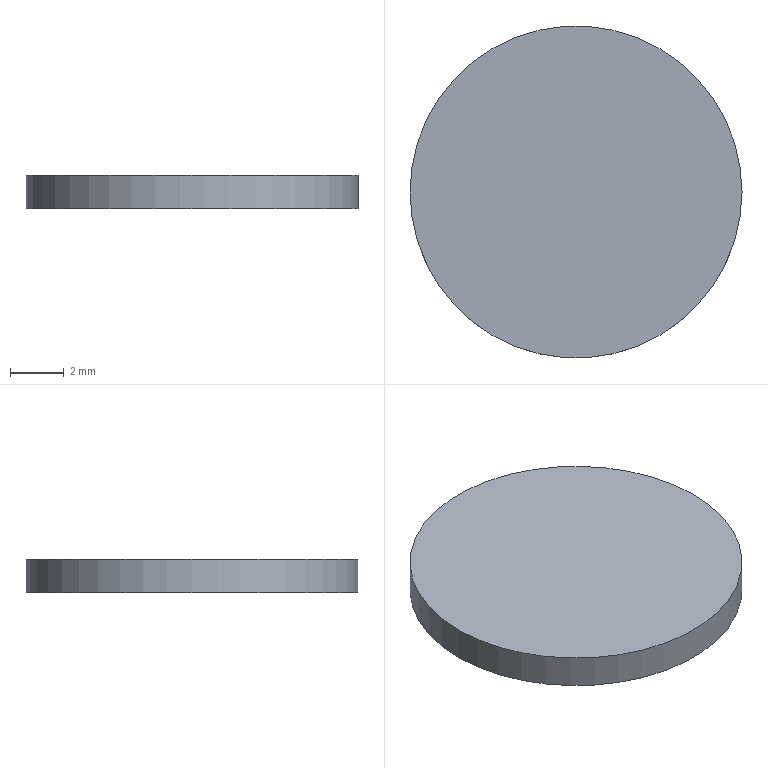Part | STEP file | gslz 2016.10.28-13_id1010_x_t | 1 solid | 3 faces | box 12.3 x 12.3 x 1.25 mm | volume 148.529 mm3 | plane 2 | cylinder 1 | commonest cylinder face diameters 12.3 x1
STEP:
#1=CARTESIAN_POINT('',(0.,0.,0.));
#2=DIRECTION('',(0.,0.,1.));
#3=DIRECTION('',(1.,0.,0.));
#4=AXIS2_PLACEMENT_3D('',#1,#2,#3);
#5=CARTESIAN_POINT('',(-1326.404,-254.,1.25));
#6=VERTEX_POINT('',#5);
#7=CARTESIAN_POINT('',(-1332.554,-254.,1.25));
#8=DIRECTION('',(0.,0.,1.));
#9=DIRECTION('',(1.,0.,0.));
#10=AXIS2_PLACEMENT_3D('',#7,#8,#9);
#11=CIRCLE('',#10,6.15);
#12=CARTESIAN_POINT('',(-1332.554,-254.,2.5));
#13=DIRECTION('',(0.,0.,-1.));
#14=DIRECTION('',(-1.,0.,0.));
#15=AXIS2_PLACEMENT_3D('',#12,#13,#14);
#16=CYLINDRICAL_SURFACE('',#15,6.15);
#17=CARTESIAN_POINT('',(9.425,1.25));
#18=DIRECTION('',(-1.,0.));
#19=VECTOR('',#18,1.);
#20=LINE('',#17,#19);
#21=(GEOMETRIC_REPRESENTATION_CONTEXT(2)PARAMETRIC_REPRESENTATION_CONTEXT()REPRESENTATION_CONTEXT('',''));
#22=DEFINITIONAL_REPRESENTATION('',(#20),#21);
#23=PCURVE('',#16,#22);
#24=CARTESIAN_POINT('',(-1332.554,-254.,1.25));
#25=DIRECTION('',(0.,0.,1.));
#26=DIRECTION('',(1.,0.,0.));
#27=AXIS2_PLACEMENT_3D('',#24,#25,#26);
#28=PLANE('',#27);
#29=CARTESIAN_POINT('',(0.,0.));
#30=DIRECTION('',(1.,0.));
#31=AXIS2_PLACEMENT_2D('',#29,#30);
#32=CIRCLE('',#31,6.15);
#33=(GEOMETRIC_REPRESENTATION_CONTEXT(2)PARAMETRIC_REPRESENTATION_CONTEXT()REPRESENTATION_CONTEXT('',''));
#34=DEFINITIONAL_REPRESENTATION('',(#32),#33);
#35=PCURVE('',#28,#34);
#36=SURFACE_CURVE('',#11,(#23,#35),.PCURVE_S1.);
#37=EDGE_CURVE('',#6,#6,#36,.T.);
#38=ORIENTED_EDGE('',*,*,#37,.F.);
#39=CARTESIAN_POINT('',(-1326.404,-254.,0.));
#40=VERTEX_POINT('',#39);
#41=CARTESIAN_POINT('',(-1326.404,-254.,1.25));
#42=CARTESIAN_POINT('',(-1326.404,-254.,0.));
#43=B_SPLINE_CURVE_WITH_KNOTS('',1,(#41,#42),.UNSPECIFIED.,.F.,.F.,(2,2),(1.25,2.5),.PIECEWISE_BEZIER_KNOTS.);
#44=CARTESIAN_POINT('',(9.425,0.));
#45=DIRECTION('',(0.,1.));
#46=VECTOR('',#45,1.);
#47=LINE('',#44,#46);
#48=(GEOMETRIC_REPRESENTATION_CONTEXT(2)PARAMETRIC_REPRESENTATION_CONTEXT()REPRESENTATION_CONTEXT('',''));
#49=DEFINITIONAL_REPRESENTATION('',(#47),#48);
#50=PCURVE('',#16,#49);
#51=CARTESIAN_POINT('',(3.142,0.));
#52=DIRECTION('',(0.,1.));
#53=VECTOR('',#52,1.);
#54=LINE('',#51,#53);
#55=(GEOMETRIC_REPRESENTATION_CONTEXT(2)PARAMETRIC_REPRESENTATION_CONTEXT()REPRESENTATION_CONTEXT('',''));
#56=DEFINITIONAL_REPRESENTATION('',(#54),#55);
#57=PCURVE('',#16,#56);
#58=SEAM_CURVE('',#43,(#50,#57),.PCURVE_S1.);
#59=EDGE_CURVE('',#6,#40,#58,.T.);
#60=ORIENTED_EDGE('',*,*,#59,.T.);
#61=CARTESIAN_POINT('',(-1332.554,-254.,0.));
#62=DIRECTION('',(0.,0.,1.));
#63=DIRECTION('',(1.,0.,0.));
#64=AXIS2_PLACEMENT_3D('',#61,#62,#63);
#65=CIRCLE('',#64,6.15);
#66=CARTESIAN_POINT('',(9.425,2.5));
#67=DIRECTION('',(-1.,0.));
#68=VECTOR('',#67,1.);
#69=LINE('',#66,#68);
#70=(GEOMETRIC_REPRESENTATION_CONTEXT(2)PARAMETRIC_REPRESENTATION_CONTEXT()REPRESENTATION_CONTEXT('',''));
#71=DEFINITIONAL_REPRESENTATION('',(#69),#70);
#72=PCURVE('',#16,#71);
#73=CARTESIAN_POINT('',(-1332.554,-254.,0.));
#74=DIRECTION('',(0.,0.,1.));
#75=DIRECTION('',(1.,0.,0.));
#76=AXIS2_PLACEMENT_3D('',#73,#74,#75);
#77=PLANE('',#76);
#78=CARTESIAN_POINT('',(0.,0.));
#79=DIRECTION('',(1.,0.));
#80=AXIS2_PLACEMENT_2D('',#78,#79);
#81=CIRCLE('',#80,6.15);
#82=(GEOMETRIC_REPRESENTATION_CONTEXT(2)PARAMETRIC_REPRESENTATION_CONTEXT()REPRESENTATION_CONTEXT('',''));
#83=DEFINITIONAL_REPRESENTATION('',(#81),#82);
#84=PCURVE('',#77,#83);
#85=SURFACE_CURVE('',#65,(#72,#84),.PCURVE_S1.);
#86=EDGE_CURVE('',#40,#40,#85,.T.);
#87=ORIENTED_EDGE('',*,*,#86,.T.);
#88=ORIENTED_EDGE('',*,*,#59,.F.);
#89=EDGE_LOOP('',(#38,#60,#87,#88));
#90=FACE_BOUND('',#89,.T.);
#91=ADVANCED_FACE('',(#90),#16,.T.);
#92=ORIENTED_EDGE('',*,*,#37,.T.);
#93=EDGE_LOOP('',(#92));
#94=FACE_BOUND('',#93,.T.);
#95=ADVANCED_FACE('',(#94),#28,.T.);
#96=ORIENTED_EDGE('',*,*,#86,.F.);
#97=EDGE_LOOP('',(#96));
#98=FACE_BOUND('',#97,.T.);
#99=ADVANCED_FACE('',(#98),#77,.F.);
#100=CLOSED_SHELL('',(#91,#95,#99));
#101=MANIFOLD_SOLID_BREP('',#100);
#102=(LENGTH_UNIT()NAMED_UNIT(*)SI_UNIT(.MILLI.,.METRE.));
#103=UNCERTAINTY_MEASURE_WITH_UNIT(LENGTH_MEASURE(0.00001),#102,'','');
#104=(NAMED_UNIT(*)PLANE_ANGLE_UNIT()SI_UNIT($,.RADIAN.));
#105=(NAMED_UNIT(*)SI_UNIT($,.STERADIAN.)SOLID_ANGLE_UNIT());
#106=(GEOMETRIC_REPRESENTATION_CONTEXT(3)GLOBAL_UNCERTAINTY_ASSIGNED_CONTEXT((#103))GLOBAL_UNIT_ASSIGNED_CONTEXT((#102,#104,#105))REPRESENTATION_CONTEXT('',''));
#107=ADVANCED_BREP_SHAPE_REPRESENTATION('',(#4,#101),#106);